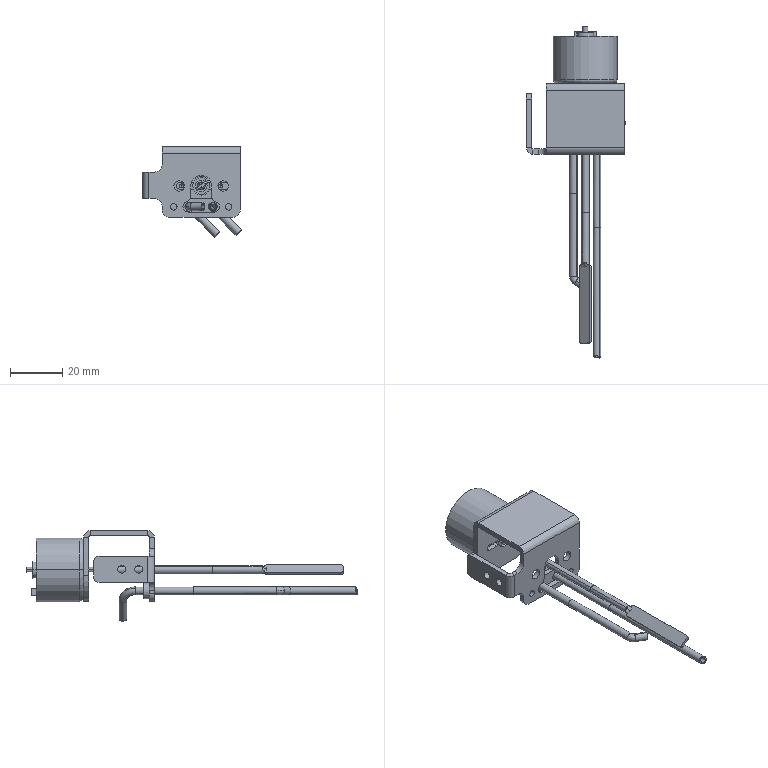Part | SolidWorks | features BaseBody 7 | 7 solids | 235 faces | box 37.96 x 127.1 x 34.667 mm | volume 14532 mm3 | cylinder 116 | plane 76 | cone 21 | torus 18 | spline 4 | commonest cylinder face diameters 3 x26 2 x20 1.6 x12 4 x11 1 x7 6 x7